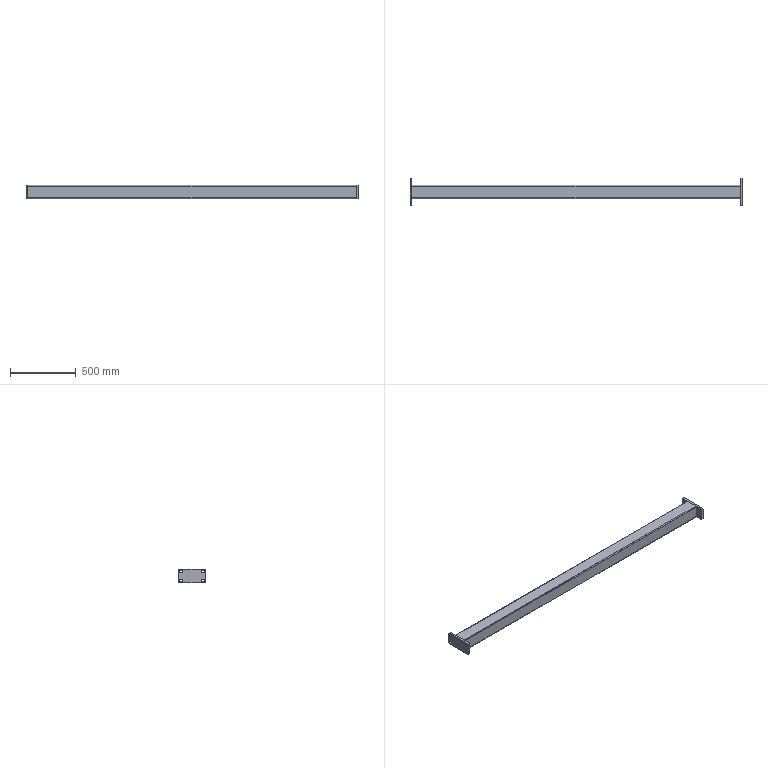Part | SolidWorks | features ICE 3, HoleWzd 2, WeldMemberFeat 2, LPattern 1, MirrorSolid 1, WeldCornerFeat 1, WeldmentFeature 1 | 3 solids | 70 faces | box 2525 x 210 x 100 mm | volume 3620734 mm3 | plane 46 | cylinder 24 | commonest cylinder face diameters 13.5 x16 6.4 x4 12.8 x4